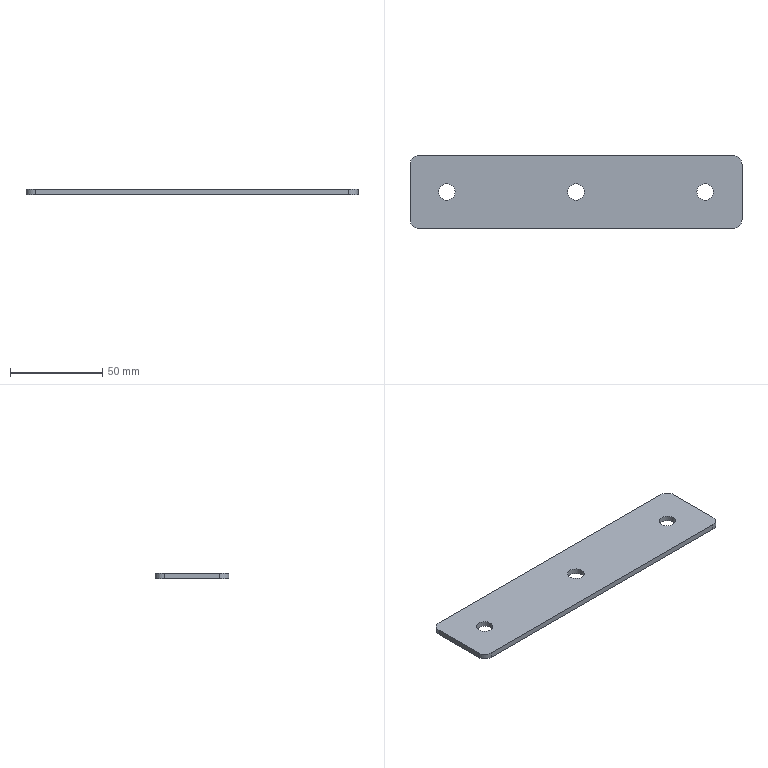Part | STEP file | 5091302 | 1 solid | 13 faces | box 180 x 40 x 3 mm | volume 20963 mm3 | cylinder 7 | plane 6 | commonest cylinder face diameters 10 x4 9 x3
STEP:
#1=CARTESIAN_POINT('',(0.,0.,0.));
#2=DIRECTION('',(0.,0.,1.));
#3=DIRECTION('',(1.,0.,0.));
#4=AXIS2_PLACEMENT_3D('',#1,#2,#3);
#5=CARTESIAN_POINT('',(-65.5,0.,3.));
#6=VERTEX_POINT('',#5);
#7=CARTESIAN_POINT('',(-70.,0.,3.));
#8=DIRECTION('',(0.,0.,1.));
#9=DIRECTION('',(1.,0.,0.));
#10=AXIS2_PLACEMENT_3D('',#7,#8,#9);
#11=CIRCLE('',#10,4.5);
#12=CARTESIAN_POINT('',(-85.,15.,3.));
#13=DIRECTION('',(0.,0.,1.));
#14=DIRECTION('',(1.,0.,0.));
#15=AXIS2_PLACEMENT_3D('',#12,#13,#14);
#16=PLANE('',#15);
#17=CARTESIAN_POINT('',(15.,-15.));
#18=DIRECTION('',(1.,0.));
#19=AXIS2_PLACEMENT_2D('',#17,#18);
#20=CIRCLE('',#19,4.5);
#21=(GEOMETRIC_REPRESENTATION_CONTEXT(2)PARAMETRIC_REPRESENTATION_CONTEXT()REPRESENTATION_CONTEXT('',''));
#22=DEFINITIONAL_REPRESENTATION('',(#20),#21);
#23=PCURVE('',#16,#22);
#24=CARTESIAN_POINT('',(-70.,0.,3.));
#25=DIRECTION('',(0.,0.,-1.));
#26=DIRECTION('',(-1.,0.,0.));
#27=AXIS2_PLACEMENT_3D('',#24,#25,#26);
#28=CYLINDRICAL_SURFACE('',#27,4.5);
#29=CARTESIAN_POINT('',(9.425,0.));
#30=DIRECTION('',(-1.,0.));
#31=VECTOR('',#30,1.);
#32=LINE('',#29,#31);
#33=(GEOMETRIC_REPRESENTATION_CONTEXT(2)PARAMETRIC_REPRESENTATION_CONTEXT()REPRESENTATION_CONTEXT('',''));
#34=DEFINITIONAL_REPRESENTATION('',(#32),#33);
#35=PCURVE('',#28,#34);
#36=SURFACE_CURVE('',#11,(#23,#35),.PCURVE_S1.);
#37=EDGE_CURVE('',#6,#6,#36,.T.);
#38=ORIENTED_EDGE('',*,*,#37,.F.);
#39=EDGE_LOOP('',(#38));
#40=FACE_BOUND('',#39,.T.);
#41=CARTESIAN_POINT('',(-85.,20.,3.));
#42=VERTEX_POINT('',#41);
#43=CARTESIAN_POINT('',(-90.,15.,3.));
#44=VERTEX_POINT('',#43);
#45=CARTESIAN_POINT('',(-85.,15.,3.));
#46=DIRECTION('',(0.,0.,1.));
#47=DIRECTION('',(1.,0.,0.));
#48=AXIS2_PLACEMENT_3D('',#45,#46,#47);
#49=CIRCLE('',#48,5.);
#50=CARTESIAN_POINT('',(0.,0.));
#51=DIRECTION('',(1.,0.));
#52=AXIS2_PLACEMENT_2D('',#50,#51);
#53=CIRCLE('',#52,5.);
#54=(GEOMETRIC_REPRESENTATION_CONTEXT(2)PARAMETRIC_REPRESENTATION_CONTEXT()REPRESENTATION_CONTEXT('',''));
#55=DEFINITIONAL_REPRESENTATION('',(#53),#54);
#56=PCURVE('',#16,#55);
#57=CARTESIAN_POINT('',(-85.,15.,3.));
#58=DIRECTION('',(0.,0.,-1.));
#59=DIRECTION('',(-1.,0.,0.));
#60=AXIS2_PLACEMENT_3D('',#57,#58,#59);
#61=CYLINDRICAL_SURFACE('',#60,5.);
#62=CARTESIAN_POINT('',(3.142,0.));
#63=DIRECTION('',(-1.,0.));
#64=VECTOR('',#63,1.);
#65=LINE('',#62,#64);
#66=(GEOMETRIC_REPRESENTATION_CONTEXT(2)PARAMETRIC_REPRESENTATION_CONTEXT()REPRESENTATION_CONTEXT('',''));
#67=DEFINITIONAL_REPRESENTATION('',(#65),#66);
#68=PCURVE('',#61,#67);
#69=SURFACE_CURVE('',#49,(#56,#68),.PCURVE_S1.);
#70=EDGE_CURVE('',#42,#44,#69,.T.);
#71=ORIENTED_EDGE('',*,*,#70,.T.);
#72=CARTESIAN_POINT('',(-90.,-15.,3.));
#73=VERTEX_POINT('',#72);
#74=CARTESIAN_POINT('',(-90.,15.,3.));
#75=DIRECTION('',(0.,-1.,0.));
#76=VECTOR('',#75,1.);
#77=LINE('',#74,#76);
#78=CARTESIAN_POINT('',(-5.,0.));
#79=DIRECTION('',(0.,-1.));
#80=VECTOR('',#79,1.);
#81=LINE('',#78,#80);
#82=(GEOMETRIC_REPRESENTATION_CONTEXT(2)PARAMETRIC_REPRESENTATION_CONTEXT()REPRESENTATION_CONTEXT('',''));
#83=DEFINITIONAL_REPRESENTATION('',(#81),#82);
#84=PCURVE('',#16,#83);
#85=CARTESIAN_POINT('',(-90.,15.,3.));
#86=DIRECTION('',(1.,0.,0.));
#87=DIRECTION('',(0.,0.,-1.));
#88=AXIS2_PLACEMENT_3D('',#85,#86,#87);
#89=PLANE('',#88);
#90=CARTESIAN_POINT('',(0.,0.));
#91=DIRECTION('',(0.,-1.));
#92=VECTOR('',#91,1.);
#93=LINE('',#90,#92);
#94=(GEOMETRIC_REPRESENTATION_CONTEXT(2)PARAMETRIC_REPRESENTATION_CONTEXT()REPRESENTATION_CONTEXT('',''));
#95=DEFINITIONAL_REPRESENTATION('',(#93),#94);
#96=PCURVE('',#89,#95);
#97=SURFACE_CURVE('',#77,(#84,#96),.PCURVE_S1.);
#98=EDGE_CURVE('',#44,#73,#97,.T.);
#99=ORIENTED_EDGE('',*,*,#98,.T.);
#100=CARTESIAN_POINT('',(-85.,-20.,3.));
#101=VERTEX_POINT('',#100);
#102=CARTESIAN_POINT('',(-85.,-15.,3.));
#103=DIRECTION('',(0.,0.,1.));
#104=DIRECTION('',(1.,0.,0.));
#105=AXIS2_PLACEMENT_3D('',#102,#103,#104);
#106=CIRCLE('',#105,5.);
#107=CARTESIAN_POINT('',(0.,-30.));
#108=DIRECTION('',(1.,0.));
#109=AXIS2_PLACEMENT_2D('',#107,#108);
#110=CIRCLE('',#109,5.);
#111=(GEOMETRIC_REPRESENTATION_CONTEXT(2)PARAMETRIC_REPRESENTATION_CONTEXT()REPRESENTATION_CONTEXT('',''));
#112=DEFINITIONAL_REPRESENTATION('',(#110),#111);
#113=PCURVE('',#16,#112);
#114=CARTESIAN_POINT('',(-85.,-15.,3.));
#115=DIRECTION('',(0.,0.,-1.));
#116=DIRECTION('',(-1.,0.,0.));
#117=AXIS2_PLACEMENT_3D('',#114,#115,#116);
#118=CYLINDRICAL_SURFACE('',#117,5.);
#119=CARTESIAN_POINT('',(9.425,0.));
#120=DIRECTION('',(-1.,0.));
#121=VECTOR('',#120,1.);
#122=LINE('',#119,#121);
#123=(GEOMETRIC_REPRESENTATION_CONTEXT(2)PARAMETRIC_REPRESENTATION_CONTEXT()REPRESENTATION_CONTEXT('',''));
#124=DEFINITIONAL_REPRESENTATION('',(#122),#123);
#125=PCURVE('',#118,#124);
#126=SURFACE_CURVE('',#106,(#113,#125),.PCURVE_S1.);
#127=EDGE_CURVE('',#73,#101,#126,.T.);
#128=ORIENTED_EDGE('',*,*,#127,.T.);
#129=CARTESIAN_POINT('',(85.,-20.,3.));
#130=VERTEX_POINT('',#129);
#131=CARTESIAN_POINT('',(-85.,-20.,3.));
#132=DIRECTION('',(1.,0.,0.));
#133=VECTOR('',#132,1.);
#134=LINE('',#131,#133);
#135=CARTESIAN_POINT('',(0.,-35.));
#136=DIRECTION('',(1.,0.));
#137=VECTOR('',#136,1.);
#138=LINE('',#135,#137);
#139=(GEOMETRIC_REPRESENTATION_CONTEXT(2)PARAMETRIC_REPRESENTATION_CONTEXT()REPRESENTATION_CONTEXT('',''));
#140=DEFINITIONAL_REPRESENTATION('',(#138),#139);
#141=PCURVE('',#16,#140);
#142=CARTESIAN_POINT('',(-85.,-20.,3.));
#143=DIRECTION('',(0.,1.,0.));
#144=DIRECTION('',(0.,0.,1.));
#145=AXIS2_PLACEMENT_3D('',#142,#143,#144);
#146=PLANE('',#145);
#147=CARTESIAN_POINT('',(0.,0.));
#148=DIRECTION('',(0.,1.));
#149=VECTOR('',#148,1.);
#150=LINE('',#147,#149);
#151=(GEOMETRIC_REPRESENTATION_CONTEXT(2)PARAMETRIC_REPRESENTATION_CONTEXT()REPRESENTATION_CONTEXT('',''));
#152=DEFINITIONAL_REPRESENTATION('',(#150),#151);
#153=PCURVE('',#146,#152);
#154=SURFACE_CURVE('',#134,(#141,#153),.PCURVE_S1.);
#155=EDGE_CURVE('',#101,#130,#154,.T.);
#156=ORIENTED_EDGE('',*,*,#155,.T.);
#157=CARTESIAN_POINT('',(90.,-15.,3.));
#158=VERTEX_POINT('',#157);
#159=CARTESIAN_POINT('',(85.,-15.,3.));
#160=DIRECTION('',(0.,0.,1.));
#161=DIRECTION('',(1.,0.,0.));
#162=AXIS2_PLACEMENT_3D('',#159,#160,#161);
#163=CIRCLE('',#162,5.);
#164=CARTESIAN_POINT('',(170.,-30.));
#165=DIRECTION('',(1.,0.));
#166=AXIS2_PLACEMENT_2D('',#164,#165);
#167=CIRCLE('',#166,5.);
#168=(GEOMETRIC_REPRESENTATION_CONTEXT(2)PARAMETRIC_REPRESENTATION_CONTEXT()REPRESENTATION_CONTEXT('',''));
#169=DEFINITIONAL_REPRESENTATION('',(#167),#168);
#170=PCURVE('',#16,#169);
#171=CARTESIAN_POINT('',(85.,-15.,3.));
#172=DIRECTION('',(0.,0.,-1.));
#173=DIRECTION('',(-1.,0.,0.));
#174=AXIS2_PLACEMENT_3D('',#171,#172,#173);
#175=CYLINDRICAL_SURFACE('',#174,5.);
#176=CARTESIAN_POINT('',(9.425,0.));
#177=DIRECTION('',(-1.,0.));
#178=VECTOR('',#177,1.);
#179=LINE('',#176,#178);
#180=(GEOMETRIC_REPRESENTATION_CONTEXT(2)PARAMETRIC_REPRESENTATION_CONTEXT()REPRESENTATION_CONTEXT('',''));
#181=DEFINITIONAL_REPRESENTATION('',(#179),#180);
#182=PCURVE('',#175,#181);
#183=SURFACE_CURVE('',#163,(#170,#182),.PCURVE_S1.);
#184=EDGE_CURVE('',#130,#158,#183,.T.);
#185=ORIENTED_EDGE('',*,*,#184,.T.);
#186=CARTESIAN_POINT('',(90.,15.,3.));
#187=VERTEX_POINT('',#186);
#188=CARTESIAN_POINT('',(90.,15.,3.));
#189=DIRECTION('',(0.,1.,0.));
#190=VECTOR('',#189,1.);
#191=LINE('',#188,#190);
#192=CARTESIAN_POINT('',(175.,0.));
#193=DIRECTION('',(0.,1.));
#194=VECTOR('',#193,1.);
#195=LINE('',#192,#194);
#196=(GEOMETRIC_REPRESENTATION_CONTEXT(2)PARAMETRIC_REPRESENTATION_CONTEXT()REPRESENTATION_CONTEXT('',''));
#197=DEFINITIONAL_REPRESENTATION('',(#195),#196);
#198=PCURVE('',#16,#197);
#199=CARTESIAN_POINT('',(90.,15.,3.));
#200=DIRECTION('',(-1.,0.,0.));
#201=DIRECTION('',(0.,0.,1.));
#202=AXIS2_PLACEMENT_3D('',#199,#200,#201);
#203=PLANE('',#202);
#204=CARTESIAN_POINT('',(0.,0.));
#205=DIRECTION('',(0.,1.));
#206=VECTOR('',#205,1.);
#207=LINE('',#204,#206);
#208=(GEOMETRIC_REPRESENTATION_CONTEXT(2)PARAMETRIC_REPRESENTATION_CONTEXT()REPRESENTATION_CONTEXT('',''));
#209=DEFINITIONAL_REPRESENTATION('',(#207),#208);
#210=PCURVE('',#203,#209);
#211=SURFACE_CURVE('',#191,(#198,#210),.PCURVE_S1.);
#212=EDGE_CURVE('',#158,#187,#211,.T.);
#213=ORIENTED_EDGE('',*,*,#212,.T.);
#214=CARTESIAN_POINT('',(85.,20.,3.));
#215=VERTEX_POINT('',#214);
#216=CARTESIAN_POINT('',(85.,15.,3.));
#217=DIRECTION('',(0.,0.,1.));
#218=DIRECTION('',(-1.,0.,0.));
#219=AXIS2_PLACEMENT_3D('',#216,#217,#218);
#220=CIRCLE('',#219,5.);
#221=CARTESIAN_POINT('',(170.,0.));
#222=DIRECTION('',(-1.,0.));
#223=AXIS2_PLACEMENT_2D('',#221,#222);
#224=CIRCLE('',#223,5.);
#225=(GEOMETRIC_REPRESENTATION_CONTEXT(2)PARAMETRIC_REPRESENTATION_CONTEXT()REPRESENTATION_CONTEXT('',''));
#226=DEFINITIONAL_REPRESENTATION('',(#224),#225);
#227=PCURVE('',#16,#226);
#228=CARTESIAN_POINT('',(85.,15.,3.));
#229=DIRECTION('',(0.,0.,-1.));
#230=DIRECTION('',(-1.,0.,0.));
#231=AXIS2_PLACEMENT_3D('',#228,#229,#230);
#232=CYLINDRICAL_SURFACE('',#231,5.);
#233=CARTESIAN_POINT('',(6.283,0.));
#234=DIRECTION('',(-1.,0.));
#235=VECTOR('',#234,1.);
#236=LINE('',#233,#235);
#237=(GEOMETRIC_REPRESENTATION_CONTEXT(2)PARAMETRIC_REPRESENTATION_CONTEXT()REPRESENTATION_CONTEXT('',''));
#238=DEFINITIONAL_REPRESENTATION('',(#236),#237);
#239=PCURVE('',#232,#238);
#240=SURFACE_CURVE('',#220,(#227,#239),.PCURVE_S1.);
#241=EDGE_CURVE('',#187,#215,#240,.T.);
#242=ORIENTED_EDGE('',*,*,#241,.T.);
#243=CARTESIAN_POINT('',(-85.,20.,3.));
#244=DIRECTION('',(-1.,0.,0.));
#245=VECTOR('',#244,1.);
#246=LINE('',#243,#245);
#247=CARTESIAN_POINT('',(0.,5.));
#248=DIRECTION('',(-1.,0.));
#249=VECTOR('',#248,1.);
#250=LINE('',#247,#249);
#251=(GEOMETRIC_REPRESENTATION_CONTEXT(2)PARAMETRIC_REPRESENTATION_CONTEXT()REPRESENTATION_CONTEXT('',''));
#252=DEFINITIONAL_REPRESENTATION('',(#250),#251);
#253=PCURVE('',#16,#252);
#254=CARTESIAN_POINT('',(-85.,20.,3.));
#255=DIRECTION('',(0.,-1.,0.));
#256=DIRECTION('',(0.,0.,-1.));
#257=AXIS2_PLACEMENT_3D('',#254,#255,#256);
#258=PLANE('',#257);
#259=CARTESIAN_POINT('',(0.,0.));
#260=DIRECTION('',(0.,-1.));
#261=VECTOR('',#260,1.);
#262=LINE('',#259,#261);
#263=(GEOMETRIC_REPRESENTATION_CONTEXT(2)PARAMETRIC_REPRESENTATION_CONTEXT()REPRESENTATION_CONTEXT('',''));
#264=DEFINITIONAL_REPRESENTATION('',(#262),#263);
#265=PCURVE('',#258,#264);
#266=SURFACE_CURVE('',#246,(#253,#265),.PCURVE_S1.);
#267=EDGE_CURVE('',#215,#42,#266,.T.);
#268=ORIENTED_EDGE('',*,*,#267,.T.);
#269=EDGE_LOOP('',(#71,#99,#128,#156,#185,#213,#242,#268));
#270=FACE_BOUND('',#269,.T.);
#271=CARTESIAN_POINT('',(74.5,0.,3.));
#272=VERTEX_POINT('',#271);
#273=CARTESIAN_POINT('',(70.,0.,3.));
#274=DIRECTION('',(0.,0.,1.));
#275=DIRECTION('',(1.,0.,0.));
#276=AXIS2_PLACEMENT_3D('',#273,#274,#275);
#277=CIRCLE('',#276,4.5);
#278=CARTESIAN_POINT('',(155.,-15.));
#279=DIRECTION('',(1.,0.));
#280=AXIS2_PLACEMENT_2D('',#278,#279);
#281=CIRCLE('',#280,4.5);
#282=(GEOMETRIC_REPRESENTATION_CONTEXT(2)PARAMETRIC_REPRESENTATION_CONTEXT()REPRESENTATION_CONTEXT('',''));
#283=DEFINITIONAL_REPRESENTATION('',(#281),#282);
#284=PCURVE('',#16,#283);
#285=CARTESIAN_POINT('',(70.,0.,3.));
#286=DIRECTION('',(0.,0.,-1.));
#287=DIRECTION('',(-1.,0.,0.));
#288=AXIS2_PLACEMENT_3D('',#285,#286,#287);
#289=CYLINDRICAL_SURFACE('',#288,4.5);
#290=CARTESIAN_POINT('',(9.425,0.));
#291=DIRECTION('',(-1.,0.));
#292=VECTOR('',#291,1.);
#293=LINE('',#290,#292);
#294=(GEOMETRIC_REPRESENTATION_CONTEXT(2)PARAMETRIC_REPRESENTATION_CONTEXT()REPRESENTATION_CONTEXT('',''));
#295=DEFINITIONAL_REPRESENTATION('',(#293),#294);
#296=PCURVE('',#289,#295);
#297=SURFACE_CURVE('',#277,(#284,#296),.PCURVE_S1.);
#298=EDGE_CURVE('',#272,#272,#297,.T.);
#299=ORIENTED_EDGE('',*,*,#298,.F.);
#300=EDGE_LOOP('',(#299));
#301=FACE_BOUND('',#300,.T.);
#302=CARTESIAN_POINT('',(4.5,0.,3.));
#303=VERTEX_POINT('',#302);
#304=CARTESIAN_POINT('',(0.,0.,3.));
#305=DIRECTION('',(0.,0.,1.));
#306=DIRECTION('',(1.,0.,0.));
#307=AXIS2_PLACEMENT_3D('',#304,#305,#306);
#308=CIRCLE('',#307,4.5);
#309=CARTESIAN_POINT('',(85.,-15.));
#310=DIRECTION('',(1.,0.));
#311=AXIS2_PLACEMENT_2D('',#309,#310);
#312=CIRCLE('',#311,4.5);
#313=(GEOMETRIC_REPRESENTATION_CONTEXT(2)PARAMETRIC_REPRESENTATION_CONTEXT()REPRESENTATION_CONTEXT('',''));
#314=DEFINITIONAL_REPRESENTATION('',(#312),#313);
#315=PCURVE('',#16,#314);
#316=CARTESIAN_POINT('',(0.,0.,3.));
#317=DIRECTION('',(0.,0.,-1.));
#318=DIRECTION('',(-1.,0.,0.));
#319=AXIS2_PLACEMENT_3D('',#316,#317,#318);
#320=CYLINDRICAL_SURFACE('',#319,4.5);
#321=CARTESIAN_POINT('',(9.425,0.));
#322=DIRECTION('',(-1.,0.));
#323=VECTOR('',#322,1.);
#324=LINE('',#321,#323);
#325=(GEOMETRIC_REPRESENTATION_CONTEXT(2)PARAMETRIC_REPRESENTATION_CONTEXT()REPRESENTATION_CONTEXT('',''));
#326=DEFINITIONAL_REPRESENTATION('',(#324),#325);
#327=PCURVE('',#320,#326);
#328=SURFACE_CURVE('',#308,(#315,#327),.PCURVE_S1.);
#329=EDGE_CURVE('',#303,#303,#328,.T.);
#330=ORIENTED_EDGE('',*,*,#329,.F.);
#331=EDGE_LOOP('',(#330));
#332=FACE_BOUND('',#331,.T.);
#333=ADVANCED_FACE('',(#40,#270,#301,#332),#16,.T.);
#334=CARTESIAN_POINT('',(-65.5,0.,0.));
#335=VERTEX_POINT('',#334);
#336=CARTESIAN_POINT('',(-70.,0.,0.));
#337=DIRECTION('',(0.,0.,1.));
#338=DIRECTION('',(1.,0.,0.));
#339=AXIS2_PLACEMENT_3D('',#336,#337,#338);
#340=CIRCLE('',#339,4.5);
#341=CARTESIAN_POINT('',(-85.,15.,0.));
#342=DIRECTION('',(0.,0.,1.));
#343=DIRECTION('',(1.,0.,0.));
#344=AXIS2_PLACEMENT_3D('',#341,#342,#343);
#345=PLANE('',#344);
#346=CARTESIAN_POINT('',(15.,-15.));
#347=DIRECTION('',(1.,0.));
#348=AXIS2_PLACEMENT_2D('',#346,#347);
#349=CIRCLE('',#348,4.5);
#350=(GEOMETRIC_REPRESENTATION_CONTEXT(2)PARAMETRIC_REPRESENTATION_CONTEXT()REPRESENTATION_CONTEXT('',''));
#351=DEFINITIONAL_REPRESENTATION('',(#349),#350);
#352=PCURVE('',#345,#351);
#353=CARTESIAN_POINT('',(9.425,3.));
#354=DIRECTION('',(-1.,0.));
#355=VECTOR('',#354,1.);
#356=LINE('',#353,#355);
#357=(GEOMETRIC_REPRESENTATION_CONTEXT(2)PARAMETRIC_REPRESENTATION_CONTEXT()REPRESENTATION_CONTEXT('',''));
#358=DEFINITIONAL_REPRESENTATION('',(#356),#357);
#359=PCURVE('',#28,#358);
#360=SURFACE_CURVE('',#340,(#352,#359),.PCURVE_S1.);
#361=EDGE_CURVE('',#335,#335,#360,.T.);
#362=ORIENTED_EDGE('',*,*,#361,.T.);
#363=EDGE_LOOP('',(#362));
#364=FACE_BOUND('',#363,.T.);
#365=CARTESIAN_POINT('',(-85.,20.,0.));
#366=VERTEX_POINT('',#365);
#367=CARTESIAN_POINT('',(-90.,15.,0.));
#368=VERTEX_POINT('',#367);
#369=CARTESIAN_POINT('',(-85.,15.,0.));
#370=DIRECTION('',(0.,0.,1.));
#371=DIRECTION('',(1.,0.,0.));
#372=AXIS2_PLACEMENT_3D('',#369,#370,#371);
#373=CIRCLE('',#372,5.);
#374=CARTESIAN_POINT('',(0.,0.));
#375=DIRECTION('',(1.,0.));
#376=AXIS2_PLACEMENT_2D('',#374,#375);
#377=CIRCLE('',#376,5.);
#378=(GEOMETRIC_REPRESENTATION_CONTEXT(2)PARAMETRIC_REPRESENTATION_CONTEXT()REPRESENTATION_CONTEXT('',''));
#379=DEFINITIONAL_REPRESENTATION('',(#377),#378);
#380=PCURVE('',#345,#379);
#381=CARTESIAN_POINT('',(3.142,3.));
#382=DIRECTION('',(-1.,0.));
#383=VECTOR('',#382,1.);
#384=LINE('',#381,#383);
#385=(GEOMETRIC_REPRESENTATION_CONTEXT(2)PARAMETRIC_REPRESENTATION_CONTEXT()REPRESENTATION_CONTEXT('',''));
#386=DEFINITIONAL_REPRESENTATION('',(#384),#385);
#387=PCURVE('',#61,#386);
#388=SURFACE_CURVE('',#373,(#380,#387),.PCURVE_S1.);
#389=EDGE_CURVE('',#366,#368,#388,.T.);
#390=ORIENTED_EDGE('',*,*,#389,.F.);
#391=CARTESIAN_POINT('',(85.,20.,0.));
#392=VERTEX_POINT('',#391);
#393=CARTESIAN_POINT('',(-85.,20.,0.));
#394=DIRECTION('',(-1.,0.,0.));
#395=VECTOR('',#394,1.);
#396=LINE('',#393,#395);
#397=CARTESIAN_POINT('',(0.,5.));
#398=DIRECTION('',(-1.,0.));
#399=VECTOR('',#398,1.);
#400=LINE('',#397,#399);
#401=(GEOMETRIC_REPRESENTATION_CONTEXT(2)PARAMETRIC_REPRESENTATION_CONTEXT()REPRESENTATION_CONTEXT('',''));
#402=DEFINITIONAL_REPRESENTATION('',(#400),#401);
#403=PCURVE('',#345,#402);
#404=CARTESIAN_POINT('',(3.,0.));
#405=DIRECTION('',(0.,-1.));
#406=VECTOR('',#405,1.);
#407=LINE('',#404,#406);
#408=(GEOMETRIC_REPRESENTATION_CONTEXT(2)PARAMETRIC_REPRESENTATION_CONTEXT()REPRESENTATION_CONTEXT('',''));
#409=DEFINITIONAL_REPRESENTATION('',(#407),#408);
#410=PCURVE('',#258,#409);
#411=SURFACE_CURVE('',#396,(#403,#410),.PCURVE_S1.);
#412=EDGE_CURVE('',#392,#366,#411,.T.);
#413=ORIENTED_EDGE('',*,*,#412,.F.);
#414=CARTESIAN_POINT('',(90.,15.,0.));
#415=VERTEX_POINT('',#414);
#416=CARTESIAN_POINT('',(85.,15.,0.));
#417=DIRECTION('',(0.,0.,1.));
#418=DIRECTION('',(-1.,0.,0.));
#419=AXIS2_PLACEMENT_3D('',#416,#417,#418);
#420=CIRCLE('',#419,5.);
#421=CARTESIAN_POINT('',(170.,0.));
#422=DIRECTION('',(-1.,0.));
#423=AXIS2_PLACEMENT_2D('',#421,#422);
#424=CIRCLE('',#423,5.);
#425=(GEOMETRIC_REPRESENTATION_CONTEXT(2)PARAMETRIC_REPRESENTATION_CONTEXT()REPRESENTATION_CONTEXT('',''));
#426=DEFINITIONAL_REPRESENTATION('',(#424),#425);
#427=PCURVE('',#345,#426);
#428=CARTESIAN_POINT('',(6.283,3.));
#429=DIRECTION('',(-1.,0.));
#430=VECTOR('',#429,1.);
#431=LINE('',#428,#430);
#432=(GEOMETRIC_REPRESENTATION_CONTEXT(2)PARAMETRIC_REPRESENTATION_CONTEXT()REPRESENTATION_CONTEXT('',''));
#433=DEFINITIONAL_REPRESENTATION('',(#431),#432);
#434=PCURVE('',#232,#433);
#435=SURFACE_CURVE('',#420,(#427,#434),.PCURVE_S1.);
#436=EDGE_CURVE('',#415,#392,#435,.T.);
#437=ORIENTED_EDGE('',*,*,#436,.F.);
#438=CARTESIAN_POINT('',(90.,-15.,0.));
#439=VERTEX_POINT('',#438);
#440=CARTESIAN_POINT('',(90.,15.,0.));
#441=DIRECTION('',(0.,1.,0.));
#442=VECTOR('',#441,1.);
#443=LINE('',#440,#442);
#444=CARTESIAN_POINT('',(175.,0.));
#445=DIRECTION('',(0.,1.));
#446=VECTOR('',#445,1.);
#447=LINE('',#444,#446);
#448=(GEOMETRIC_REPRESENTATION_CONTEXT(2)PARAMETRIC_REPRESENTATION_CONTEXT()REPRESENTATION_CONTEXT('',''));
#449=DEFINITIONAL_REPRESENTATION('',(#447),#448);
#450=PCURVE('',#345,#449);
#451=CARTESIAN_POINT('',(-3.,0.));
#452=DIRECTION('',(0.,1.));
#453=VECTOR('',#452,1.);
#454=LINE('',#451,#453);
#455=(GEOMETRIC_REPRESENTATION_CONTEXT(2)PARAMETRIC_REPRESENTATION_CONTEXT()REPRESENTATION_CONTEXT('',''));
#456=DEFINITIONAL_REPRESENTATION('',(#454),#455);
#457=PCURVE('',#203,#456);
#458=SURFACE_CURVE('',#443,(#450,#457),.PCURVE_S1.);
#459=EDGE_CURVE('',#439,#415,#458,.T.);
#460=ORIENTED_EDGE('',*,*,#459,.F.);
#461=CARTESIAN_POINT('',(85.,-20.,0.));
#462=VERTEX_POINT('',#461);
#463=CARTESIAN_POINT('',(85.,-15.,0.));
#464=DIRECTION('',(0.,0.,1.));
#465=DIRECTION('',(1.,0.,0.));
#466=AXIS2_PLACEMENT_3D('',#463,#464,#465);
#467=CIRCLE('',#466,5.);
#468=CARTESIAN_POINT('',(170.,-30.));
#469=DIRECTION('',(1.,0.));
#470=AXIS2_PLACEMENT_2D('',#468,#469);
#471=CIRCLE('',#470,5.);
#472=(GEOMETRIC_REPRESENTATION_CONTEXT(2)PARAMETRIC_REPRESENTATION_CONTEXT()REPRESENTATION_CONTEXT('',''));
#473=DEFINITIONAL_REPRESENTATION('',(#471),#472);
#474=PCURVE('',#345,#473);
#475=CARTESIAN_POINT('',(9.425,3.));
#476=DIRECTION('',(-1.,0.));
#477=VECTOR('',#476,1.);
#478=LINE('',#475,#477);
#479=(GEOMETRIC_REPRESENTATION_CONTEXT(2)PARAMETRIC_REPRESENTATION_CONTEXT()REPRESENTATION_CONTEXT('',''));
#480=DEFINITIONAL_REPRESENTATION('',(#478),#479);
#481=PCURVE('',#175,#480);
#482=SURFACE_CURVE('',#467,(#474,#481),.PCURVE_S1.);
#483=EDGE_CURVE('',#462,#439,#482,.T.);
#484=ORIENTED_EDGE('',*,*,#483,.F.);
#485=CARTESIAN_POINT('',(-85.,-20.,0.));
#486=VERTEX_POINT('',#485);
#487=CARTESIAN_POINT('',(-85.,-20.,0.));
#488=DIRECTION('',(1.,0.,0.));
#489=VECTOR('',#488,1.);
#490=LINE('',#487,#489);
#491=CARTESIAN_POINT('',(0.,-35.));
#492=DIRECTION('',(1.,0.));
#493=VECTOR('',#492,1.);
#494=LINE('',#491,#493);
#495=(GEOMETRIC_REPRESENTATION_CONTEXT(2)PARAMETRIC_REPRESENTATION_CONTEXT()REPRESENTATION_CONTEXT('',''));
#496=DEFINITIONAL_REPRESENTATION('',(#494),#495);
#497=PCURVE('',#345,#496);
#498=CARTESIAN_POINT('',(-3.,0.));
#499=DIRECTION('',(0.,1.));
#500=VECTOR('',#499,1.);
#501=LINE('',#498,#500);
#502=(GEOMETRIC_REPRESENTATION_CONTEXT(2)PARAMETRIC_REPRESENTATION_CONTEXT()REPRESENTATION_CONTEXT('',''));
#503=DEFINITIONAL_REPRESENTATION('',(#501),#502);
#504=PCURVE('',#146,#503);
#505=SURFACE_CURVE('',#490,(#497,#504),.PCURVE_S1.);
#506=EDGE_CURVE('',#486,#462,#505,.T.);
#507=ORIENTED_EDGE('',*,*,#506,.F.);
#508=CARTESIAN_POINT('',(-90.,-15.,0.));
#509=VERTEX_POINT('',#508);
#510=CARTESIAN_POINT('',(-85.,-15.,0.));
#511=DIRECTION('',(0.,0.,1.));
#512=DIRECTION('',(1.,0.,0.));
#513=AXIS2_PLACEMENT_3D('',#510,#511,#512);
#514=CIRCLE('',#513,5.);
#515=CARTESIAN_POINT('',(0.,-30.));
#516=DIRECTION('',(1.,0.));
#517=AXIS2_PLACEMENT_2D('',#515,#516);
#518=CIRCLE('',#517,5.);
#519=(GEOMETRIC_REPRESENTATION_CONTEXT(2)PARAMETRIC_REPRESENTATION_CONTEXT()REPRESENTATION_CONTEXT('',''));
#520=DEFINITIONAL_REPRESENTATION('',(#518),#519);
#521=PCURVE('',#345,#520);
#522=CARTESIAN_POINT('',(9.425,3.));
#523=DIRECTION('',(-1.,0.));
#524=VECTOR('',#523,1.);
#525=LINE('',#522,#524);
#526=(GEOMETRIC_REPRESENTATION_CONTEXT(2)PARAMETRIC_REPRESENTATION_CONTEXT()REPRESENTATION_CONTEXT('',''));
#527=DEFINITIONAL_REPRESENTATION('',(#525),#526);
#528=PCURVE('',#118,#527);
#529=SURFACE_CURVE('',#514,(#521,#528),.PCURVE_S1.);
#530=EDGE_CURVE('',#509,#486,#529,.T.);
#531=ORIENTED_EDGE('',*,*,#530,.F.);
#532=CARTESIAN_POINT('',(-90.,15.,0.));
#533=DIRECTION('',(0.,-1.,0.));
#534=VECTOR('',#533,1.);
#535=LINE('',#532,#534);
#536=CARTESIAN_POINT('',(-5.,0.));
#537=DIRECTION('',(0.,-1.));
#538=VECTOR('',#537,1.);
#539=LINE('',#536,#538);
#540=(GEOMETRIC_REPRESENTATION_CONTEXT(2)PARAMETRIC_REPRESENTATION_CONTEXT()REPRESENTATION_CONTEXT('',''));
#541=DEFINITIONAL_REPRESENTATION('',(#539),#540);
#542=PCURVE('',#345,#541);
#543=CARTESIAN_POINT('',(3.,0.));
#544=DIRECTION('',(0.,-1.));
#545=VECTOR('',#544,1.);
#546=LINE('',#543,#545);
#547=(GEOMETRIC_REPRESENTATION_CONTEXT(2)PARAMETRIC_REPRESENTATION_CONTEXT()REPRESENTATION_CONTEXT('',''));
#548=DEFINITIONAL_REPRESENTATION('',(#546),#547);
#549=PCURVE('',#89,#548);
#550=SURFACE_CURVE('',#535,(#542,#549),.PCURVE_S1.);
#551=EDGE_CURVE('',#368,#509,#550,.T.);
#552=ORIENTED_EDGE('',*,*,#551,.F.);
#553=EDGE_LOOP('',(#390,#413,#437,#460,#484,#507,#531,#552));
#554=FACE_BOUND('',#553,.T.);
#555=CARTESIAN_POINT('',(74.5,0.,0.));
#556=VERTEX_POINT('',#555);
#557=CARTESIAN_POINT('',(70.,0.,0.));
#558=DIRECTION('',(0.,0.,1.));
#559=DIRECTION('',(1.,0.,0.));
#560=AXIS2_PLACEMENT_3D('',#557,#558,#559);
#561=CIRCLE('',#560,4.5);
#562=CARTESIAN_POINT('',(155.,-15.));
#563=DIRECTION('',(1.,0.));
#564=AXIS2_PLACEMENT_2D('',#562,#563);
#565=CIRCLE('',#564,4.5);
#566=(GEOMETRIC_REPRESENTATION_CONTEXT(2)PARAMETRIC_REPRESENTATION_CONTEXT()REPRESENTATION_CONTEXT('',''));
#567=DEFINITIONAL_REPRESENTATION('',(#565),#566);
#568=PCURVE('',#345,#567);
#569=CARTESIAN_POINT('',(9.425,3.));
#570=DIRECTION('',(-1.,0.));
#571=VECTOR('',#570,1.);
#572=LINE('',#569,#571);
#573=(GEOMETRIC_REPRESENTATION_CONTEXT(2)PARAMETRIC_REPRESENTATION_CONTEXT()REPRESENTATION_CONTEXT('',''));
#574=DEFINITIONAL_REPRESENTATION('',(#572),#573);
#575=PCURVE('',#289,#574);
#576=SURFACE_CURVE('',#561,(#568,#575),.PCURVE_S1.);
#577=EDGE_CURVE('',#556,#556,#576,.T.);
#578=ORIENTED_EDGE('',*,*,#577,.T.);
#579=EDGE_LOOP('',(#578));
#580=FACE_BOUND('',#579,.T.);
#581=CARTESIAN_POINT('',(4.5,0.,0.));
#582=VERTEX_POINT('',#581);
#583=CARTESIAN_POINT('',(0.,0.,0.));
#584=DIRECTION('',(0.,0.,1.));
#585=DIRECTION('',(1.,0.,0.));
#586=AXIS2_PLACEMENT_3D('',#583,#584,#585);
#587=CIRCLE('',#586,4.5);
#588=CARTESIAN_POINT('',(85.,-15.));
#589=DIRECTION('',(1.,0.));
#590=AXIS2_PLACEMENT_2D('',#588,#589);
#591=CIRCLE('',#590,4.5);
#592=(GEOMETRIC_REPRESENTATION_CONTEXT(2)PARAMETRIC_REPRESENTATION_CONTEXT()REPRESENTATION_CONTEXT('',''));
#593=DEFINITIONAL_REPRESENTATION('',(#591),#592);
#594=PCURVE('',#345,#593);
#595=CARTESIAN_POINT('',(9.425,3.));
#596=DIRECTION('',(-1.,0.));
#597=VECTOR('',#596,1.);
#598=LINE('',#595,#597);
#599=(GEOMETRIC_REPRESENTATION_CONTEXT(2)PARAMETRIC_REPRESENTATION_CONTEXT()REPRESENTATION_CONTEXT('',''));
#600=DEFINITIONAL_REPRESENTATION('',(#598),#599);
#601=PCURVE('',#320,#600);
#602=SURFACE_CURVE('',#587,(#594,#601),.PCURVE_S1.);
#603=EDGE_CURVE('',#582,#582,#602,.T.);
#604=ORIENTED_EDGE('',*,*,#603,.T.);
#605=EDGE_LOOP('',(#604));
#606=FACE_BOUND('',#605,.T.);
#607=ADVANCED_FACE('',(#364,#554,#580,#606),#345,.F.);
#608=ORIENTED_EDGE('',*,*,#389,.T.);
#609=CARTESIAN_POINT('',(-90.,15.,3.));
#610=DIRECTION('',(0.,0.,-1.));
#611=VECTOR('',#610,1.);
#612=LINE('',#609,#611);
#613=CARTESIAN_POINT('',(0.,0.));
#614=DIRECTION('',(0.,1.));
#615=VECTOR('',#614,1.);
#616=LINE('',#613,#615);
#617=(GEOMETRIC_REPRESENTATION_CONTEXT(2)PARAMETRIC_REPRESENTATION_CONTEXT()REPRESENTATION_CONTEXT('',''));
#618=DEFINITIONAL_REPRESENTATION('',(#616),#617);
#619=PCURVE('',#61,#618);
#620=CARTESIAN_POINT('',(0.,0.));
#621=DIRECTION('',(1.,0.));
#622=VECTOR('',#621,1.);
#623=LINE('',#620,#622);
#624=(GEOMETRIC_REPRESENTATION_CONTEXT(2)PARAMETRIC_REPRESENTATION_CONTEXT()REPRESENTATION_CONTEXT('',''));
#625=DEFINITIONAL_REPRESENTATION('',(#623),#624);
#626=PCURVE('',#89,#625);
#627=SURFACE_CURVE('',#612,(#619,#626),.PCURVE_S1.);
#628=EDGE_CURVE('',#44,#368,#627,.T.);
#629=ORIENTED_EDGE('',*,*,#628,.F.);
#630=ORIENTED_EDGE('',*,*,#70,.F.);
#631=CARTESIAN_POINT('',(-85.,20.,3.));
#632=DIRECTION('',(0.,0.,-1.));
#633=VECTOR('',#632,1.);
#634=LINE('',#631,#633);
#635=CARTESIAN_POINT('',(1.571,0.));
#636=DIRECTION('',(0.,1.));
#637=VECTOR('',#636,1.);
#638=LINE('',#635,#637);
#639=(GEOMETRIC_REPRESENTATION_CONTEXT(2)PARAMETRIC_REPRESENTATION_CONTEXT()REPRESENTATION_CONTEXT('',''));
#640=DEFINITIONAL_REPRESENTATION('',(#638),#639);
#641=PCURVE('',#61,#640);
#642=CARTESIAN_POINT('',(0.,0.));
#643=DIRECTION('',(1.,0.));
#644=VECTOR('',#643,1.);
#645=LINE('',#642,#644);
#646=(GEOMETRIC_REPRESENTATION_CONTEXT(2)PARAMETRIC_REPRESENTATION_CONTEXT()REPRESENTATION_CONTEXT('',''));
#647=DEFINITIONAL_REPRESENTATION('',(#645),#646);
#648=PCURVE('',#258,#647);
#649=SURFACE_CURVE('',#634,(#641,#648),.PCURVE_S1.);
#650=EDGE_CURVE('',#42,#366,#649,.T.);
#651=ORIENTED_EDGE('',*,*,#650,.T.);
#652=EDGE_LOOP('',(#608,#629,#630,#651));
#653=FACE_BOUND('',#652,.T.);
#654=ADVANCED_FACE('',(#653),#61,.T.);
#655=ORIENTED_EDGE('',*,*,#551,.T.);
#656=CARTESIAN_POINT('',(-90.,-15.,3.));
#657=DIRECTION('',(0.,0.,-1.));
#658=VECTOR('',#657,1.);
#659=LINE('',#656,#658);
#660=CARTESIAN_POINT('',(0.,-30.));
#661=DIRECTION('',(1.,0.));
#662=VECTOR('',#661,1.);
#663=LINE('',#660,#662);
#664=(GEOMETRIC_REPRESENTATION_CONTEXT(2)PARAMETRIC_REPRESENTATION_CONTEXT()REPRESENTATION_CONTEXT('',''));
#665=DEFINITIONAL_REPRESENTATION('',(#663),#664);
#666=PCURVE('',#89,#665);
#667=CARTESIAN_POINT('',(6.283,0.));
#668=DIRECTION('',(0.,1.));
#669=VECTOR('',#668,1.);
#670=LINE('',#667,#669);
#671=(GEOMETRIC_REPRESENTATION_CONTEXT(2)PARAMETRIC_REPRESENTATION_CONTEXT()REPRESENTATION_CONTEXT('',''));
#672=DEFINITIONAL_REPRESENTATION('',(#670),#671);
#673=PCURVE('',#118,#672);
#674=SURFACE_CURVE('',#659,(#666,#673),.PCURVE_S1.);
#675=EDGE_CURVE('',#73,#509,#674,.T.);
#676=ORIENTED_EDGE('',*,*,#675,.F.);
#677=ORIENTED_EDGE('',*,*,#98,.F.);
#678=ORIENTED_EDGE('',*,*,#628,.T.);
#679=EDGE_LOOP('',(#655,#676,#677,#678));
#680=FACE_BOUND('',#679,.T.);
#681=ADVANCED_FACE('',(#680),#89,.F.);
#682=ORIENTED_EDGE('',*,*,#530,.T.);
#683=CARTESIAN_POINT('',(-85.,-20.,3.));
#684=DIRECTION('',(0.,0.,-1.));
#685=VECTOR('',#684,1.);
#686=LINE('',#683,#685);
#687=CARTESIAN_POINT('',(4.712,0.));
#688=DIRECTION('',(0.,1.));
#689=VECTOR('',#688,1.);
#690=LINE('',#687,#689);
#691=(GEOMETRIC_REPRESENTATION_CONTEXT(2)PARAMETRIC_REPRESENTATION_CONTEXT()REPRESENTATION_CONTEXT('',''));
#692=DEFINITIONAL_REPRESENTATION('',(#690),#691);
#693=PCURVE('',#118,#692);
#694=CARTESIAN_POINT('',(0.,0.));
#695=DIRECTION('',(-1.,0.));
#696=VECTOR('',#695,1.);
#697=LINE('',#694,#696);
#698=(GEOMETRIC_REPRESENTATION_CONTEXT(2)PARAMETRIC_REPRESENTATION_CONTEXT()REPRESENTATION_CONTEXT('',''));
#699=DEFINITIONAL_REPRESENTATION('',(#697),#698);
#700=PCURVE('',#146,#699);
#701=SURFACE_CURVE('',#686,(#693,#700),.PCURVE_S1.);
#702=EDGE_CURVE('',#101,#486,#701,.T.);
#703=ORIENTED_EDGE('',*,*,#702,.F.);
#704=ORIENTED_EDGE('',*,*,#127,.F.);
#705=ORIENTED_EDGE('',*,*,#675,.T.);
#706=EDGE_LOOP('',(#682,#703,#704,#705));
#707=FACE_BOUND('',#706,.T.);
#708=ADVANCED_FACE('',(#707),#118,.T.);
#709=ORIENTED_EDGE('',*,*,#506,.T.);
#710=CARTESIAN_POINT('',(85.,-20.,3.));
#711=DIRECTION('',(0.,0.,-1.));
#712=VECTOR('',#711,1.);
#713=LINE('',#710,#712);
#714=CARTESIAN_POINT('',(0.,170.));
#715=DIRECTION('',(-1.,0.));
#716=VECTOR('',#715,1.);
#717=LINE('',#714,#716);
#718=(GEOMETRIC_REPRESENTATION_CONTEXT(2)PARAMETRIC_REPRESENTATION_CONTEXT()REPRESENTATION_CONTEXT('',''));
#719=DEFINITIONAL_REPRESENTATION('',(#717),#718);
#720=PCURVE('',#146,#719);
#721=CARTESIAN_POINT('',(4.712,0.));
#722=DIRECTION('',(0.,1.));
#723=VECTOR('',#722,1.);
#724=LINE('',#721,#723);
#725=(GEOMETRIC_REPRESENTATION_CONTEXT(2)PARAMETRIC_REPRESENTATION_CONTEXT()REPRESENTATION_CONTEXT('',''));
#726=DEFINITIONAL_REPRESENTATION('',(#724),#725);
#727=PCURVE('',#175,#726);
#728=SURFACE_CURVE('',#713,(#720,#727),.PCURVE_S1.);
#729=EDGE_CURVE('',#130,#462,#728,.T.);
#730=ORIENTED_EDGE('',*,*,#729,.F.);
#731=ORIENTED_EDGE('',*,*,#155,.F.);
#732=ORIENTED_EDGE('',*,*,#702,.T.);
#733=EDGE_LOOP('',(#709,#730,#731,#732));
#734=FACE_BOUND('',#733,.T.);
#735=ADVANCED_FACE('',(#734),#146,.F.);
#736=ORIENTED_EDGE('',*,*,#483,.T.);
#737=CARTESIAN_POINT('',(90.,-15.,3.));
#738=DIRECTION('',(0.,0.,-1.));
#739=VECTOR('',#738,1.);
#740=LINE('',#737,#739);
#741=CARTESIAN_POINT('',(3.142,0.));
#742=DIRECTION('',(0.,1.));
#743=VECTOR('',#742,1.);
#744=LINE('',#741,#743);
#745=(GEOMETRIC_REPRESENTATION_CONTEXT(2)PARAMETRIC_REPRESENTATION_CONTEXT()REPRESENTATION_CONTEXT('',''));
#746=DEFINITIONAL_REPRESENTATION('',(#744),#745);
#747=PCURVE('',#175,#746);
#748=CARTESIAN_POINT('',(0.,-30.));
#749=DIRECTION('',(-1.,0.));
#750=VECTOR('',#749,1.);
#751=LINE('',#748,#750);
#752=(GEOMETRIC_REPRESENTATION_CONTEXT(2)PARAMETRIC_REPRESENTATION_CONTEXT()REPRESENTATION_CONTEXT('',''));
#753=DEFINITIONAL_REPRESENTATION('',(#751),#752);
#754=PCURVE('',#203,#753);
#755=SURFACE_CURVE('',#740,(#747,#754),.PCURVE_S1.);
#756=EDGE_CURVE('',#158,#439,#755,.T.);
#757=ORIENTED_EDGE('',*,*,#756,.F.);
#758=ORIENTED_EDGE('',*,*,#184,.F.);
#759=ORIENTED_EDGE('',*,*,#729,.T.);
#760=EDGE_LOOP('',(#736,#757,#758,#759));
#761=FACE_BOUND('',#760,.T.);
#762=ADVANCED_FACE('',(#761),#175,.T.);
#763=ORIENTED_EDGE('',*,*,#459,.T.);
#764=CARTESIAN_POINT('',(90.,15.,3.));
#765=DIRECTION('',(0.,0.,-1.));
#766=VECTOR('',#765,1.);
#767=LINE('',#764,#766);
#768=CARTESIAN_POINT('',(0.,0.));
#769=DIRECTION('',(-1.,0.));
#770=VECTOR('',#769,1.);
#771=LINE('',#768,#770);
#772=(GEOMETRIC_REPRESENTATION_CONTEXT(2)PARAMETRIC_REPRESENTATION_CONTEXT()REPRESENTATION_CONTEXT('',''));
#773=DEFINITIONAL_REPRESENTATION('',(#771),#772);
#774=PCURVE('',#203,#773);
#775=CARTESIAN_POINT('',(3.142,0.));
#776=DIRECTION('',(0.,1.));
#777=VECTOR('',#776,1.);
#778=LINE('',#775,#777);
#779=(GEOMETRIC_REPRESENTATION_CONTEXT(2)PARAMETRIC_REPRESENTATION_CONTEXT()REPRESENTATION_CONTEXT('',''));
#780=DEFINITIONAL_REPRESENTATION('',(#778),#779);
#781=PCURVE('',#232,#780);
#782=SURFACE_CURVE('',#767,(#774,#781),.PCURVE_S1.);
#783=EDGE_CURVE('',#187,#415,#782,.T.);
#784=ORIENTED_EDGE('',*,*,#783,.F.);
#785=ORIENTED_EDGE('',*,*,#212,.F.);
#786=ORIENTED_EDGE('',*,*,#756,.T.);
#787=EDGE_LOOP('',(#763,#784,#785,#786));
#788=FACE_BOUND('',#787,.T.);
#789=ADVANCED_FACE('',(#788),#203,.F.);
#790=ORIENTED_EDGE('',*,*,#436,.T.);
#791=CARTESIAN_POINT('',(85.,20.,3.));
#792=DIRECTION('',(0.,0.,-1.));
#793=VECTOR('',#792,1.);
#794=LINE('',#791,#793);
#795=CARTESIAN_POINT('',(1.571,0.));
#796=DIRECTION('',(0.,1.));
#797=VECTOR('',#796,1.);
#798=LINE('',#795,#797);
#799=(GEOMETRIC_REPRESENTATION_CONTEXT(2)PARAMETRIC_REPRESENTATION_CONTEXT()REPRESENTATION_CONTEXT('',''));
#800=DEFINITIONAL_REPRESENTATION('',(#798),#799);
#801=PCURVE('',#232,#800);
#802=CARTESIAN_POINT('',(0.,170.));
#803=DIRECTION('',(1.,0.));
#804=VECTOR('',#803,1.);
#805=LINE('',#802,#804);
#806=(GEOMETRIC_REPRESENTATION_CONTEXT(2)PARAMETRIC_REPRESENTATION_CONTEXT()REPRESENTATION_CONTEXT('',''));
#807=DEFINITIONAL_REPRESENTATION('',(#805),#806);
#808=PCURVE('',#258,#807);
#809=SURFACE_CURVE('',#794,(#801,#808),.PCURVE_S1.);
#810=EDGE_CURVE('',#215,#392,#809,.T.);
#811=ORIENTED_EDGE('',*,*,#810,.F.);
#812=ORIENTED_EDGE('',*,*,#241,.F.);
#813=ORIENTED_EDGE('',*,*,#783,.T.);
#814=EDGE_LOOP('',(#790,#811,#812,#813));
#815=FACE_BOUND('',#814,.T.);
#816=ADVANCED_FACE('',(#815),#232,.T.);
#817=ORIENTED_EDGE('',*,*,#412,.T.);
#818=ORIENTED_EDGE('',*,*,#650,.F.);
#819=ORIENTED_EDGE('',*,*,#267,.F.);
#820=ORIENTED_EDGE('',*,*,#810,.T.);
#821=EDGE_LOOP('',(#817,#818,#819,#820));
#822=FACE_BOUND('',#821,.T.);
#823=ADVANCED_FACE('',(#822),#258,.F.);
#824=ORIENTED_EDGE('',*,*,#298,.F.);
#825=CARTESIAN_POINT('',(74.5,0.,3.));
#826=CARTESIAN_POINT('',(74.5,0.,0.));
#827=B_SPLINE_CURVE_WITH_KNOTS('',1,(#825,#826),.UNSPECIFIED.,.F.,.F.,(2,2),(0.,3.),.PIECEWISE_BEZIER_KNOTS.);
#828=CARTESIAN_POINT('',(9.425,0.));
#829=DIRECTION('',(0.,1.));
#830=VECTOR('',#829,1.);
#831=LINE('',#828,#830);
#832=(GEOMETRIC_REPRESENTATION_CONTEXT(2)PARAMETRIC_REPRESENTATION_CONTEXT()REPRESENTATION_CONTEXT('',''));
#833=DEFINITIONAL_REPRESENTATION('',(#831),#832);
#834=PCURVE('',#289,#833);
#835=CARTESIAN_POINT('',(3.142,0.));
#836=DIRECTION('',(0.,1.));
#837=VECTOR('',#836,1.);
#838=LINE('',#835,#837);
#839=(GEOMETRIC_REPRESENTATION_CONTEXT(2)PARAMETRIC_REPRESENTATION_CONTEXT()REPRESENTATION_CONTEXT('',''));
#840=DEFINITIONAL_REPRESENTATION('',(#838),#839);
#841=PCURVE('',#289,#840);
#842=SEAM_CURVE('',#827,(#834,#841),.PCURVE_S1.);
#843=EDGE_CURVE('',#272,#556,#842,.T.);
#844=ORIENTED_EDGE('',*,*,#843,.T.);
#845=ORIENTED_EDGE('',*,*,#577,.T.);
#846=ORIENTED_EDGE('',*,*,#843,.F.);
#847=EDGE_LOOP('',(#824,#844,#845,#846));
#848=FACE_BOUND('',#847,.F.);
#849=ADVANCED_FACE('',(#848),#289,.F.);
#850=ORIENTED_EDGE('',*,*,#37,.F.);
#851=CARTESIAN_POINT('',(-65.5,0.,3.));
#852=CARTESIAN_POINT('',(-65.5,0.,0.));
#853=B_SPLINE_CURVE_WITH_KNOTS('',1,(#851,#852),.UNSPECIFIED.,.F.,.F.,(2,2),(0.,3.),.PIECEWISE_BEZIER_KNOTS.);
#854=CARTESIAN_POINT('',(9.425,0.));
#855=DIRECTION('',(0.,1.));
#856=VECTOR('',#855,1.);
#857=LINE('',#854,#856);
#858=(GEOMETRIC_REPRESENTATION_CONTEXT(2)PARAMETRIC_REPRESENTATION_CONTEXT()REPRESENTATION_CONTEXT('',''));
#859=DEFINITIONAL_REPRESENTATION('',(#857),#858);
#860=PCURVE('',#28,#859);
#861=CARTESIAN_POINT('',(3.142,0.));
#862=DIRECTION('',(0.,1.));
#863=VECTOR('',#862,1.);
#864=LINE('',#861,#863);
#865=(GEOMETRIC_REPRESENTATION_CONTEXT(2)PARAMETRIC_REPRESENTATION_CONTEXT()REPRESENTATION_CONTEXT('',''));
#866=DEFINITIONAL_REPRESENTATION('',(#864),#865);
#867=PCURVE('',#28,#866);
#868=SEAM_CURVE('',#853,(#860,#867),.PCURVE_S1.);
#869=EDGE_CURVE('',#6,#335,#868,.T.);
#870=ORIENTED_EDGE('',*,*,#869,.T.);
#871=ORIENTED_EDGE('',*,*,#361,.T.);
#872=ORIENTED_EDGE('',*,*,#869,.F.);
#873=EDGE_LOOP('',(#850,#870,#871,#872));
#874=FACE_BOUND('',#873,.F.);
#875=ADVANCED_FACE('',(#874),#28,.F.);
#876=ORIENTED_EDGE('',*,*,#329,.F.);
#877=CARTESIAN_POINT('',(4.5,0.,3.));
#878=CARTESIAN_POINT('',(4.5,0.,0.));
#879=B_SPLINE_CURVE_WITH_KNOTS('',1,(#877,#878),.UNSPECIFIED.,.F.,.F.,(2,2),(0.,3.),.PIECEWISE_BEZIER_KNOTS.);
#880=CARTESIAN_POINT('',(9.425,0.));
#881=DIRECTION('',(0.,1.));
#882=VECTOR('',#881,1.);
#883=LINE('',#880,#882);
#884=(GEOMETRIC_REPRESENTATION_CONTEXT(2)PARAMETRIC_REPRESENTATION_CONTEXT()REPRESENTATION_CONTEXT('',''));
#885=DEFINITIONAL_REPRESENTATION('',(#883),#884);
#886=PCURVE('',#320,#885);
#887=CARTESIAN_POINT('',(3.142,0.));
#888=DIRECTION('',(0.,1.));
#889=VECTOR('',#888,1.);
#890=LINE('',#887,#889);
#891=(GEOMETRIC_REPRESENTATION_CONTEXT(2)PARAMETRIC_REPRESENTATION_CONTEXT()REPRESENTATION_CONTEXT('',''));
#892=DEFINITIONAL_REPRESENTATION('',(#890),#891);
#893=PCURVE('',#320,#892);
#894=SEAM_CURVE('',#879,(#886,#893),.PCURVE_S1.);
#895=EDGE_CURVE('',#303,#582,#894,.T.);
#896=ORIENTED_EDGE('',*,*,#895,.T.);
#897=ORIENTED_EDGE('',*,*,#603,.T.);
#898=ORIENTED_EDGE('',*,*,#895,.F.);
#899=EDGE_LOOP('',(#876,#896,#897,#898));
#900=FACE_BOUND('',#899,.F.);
#901=ADVANCED_FACE('',(#900),#320,.F.);
#902=CLOSED_SHELL('',(#333,#607,#654,#681,#708,#735,#762,#789,#816,#823,#849,#875,#901));
#903=MANIFOLD_SOLID_BREP('',#902);
#904=(LENGTH_UNIT()NAMED_UNIT(*)SI_UNIT(.MILLI.,.METRE.));
#905=UNCERTAINTY_MEASURE_WITH_UNIT(LENGTH_MEASURE(0.000002),#904,'','');
#906=(NAMED_UNIT(*)PLANE_ANGLE_UNIT()SI_UNIT($,.RADIAN.));
#907=(NAMED_UNIT(*)SI_UNIT($,.STERADIAN.)SOLID_ANGLE_UNIT());
#908=(GEOMETRIC_REPRESENTATION_CONTEXT(3)GLOBAL_UNCERTAINTY_ASSIGNED_CONTEXT((#905))GLOBAL_UNIT_ASSIGNED_CONTEXT((#904,#906,#907))REPRESENTATION_CONTEXT('',''));
#909=ADVANCED_BREP_SHAPE_REPRESENTATION('',(#4,#903),#908);